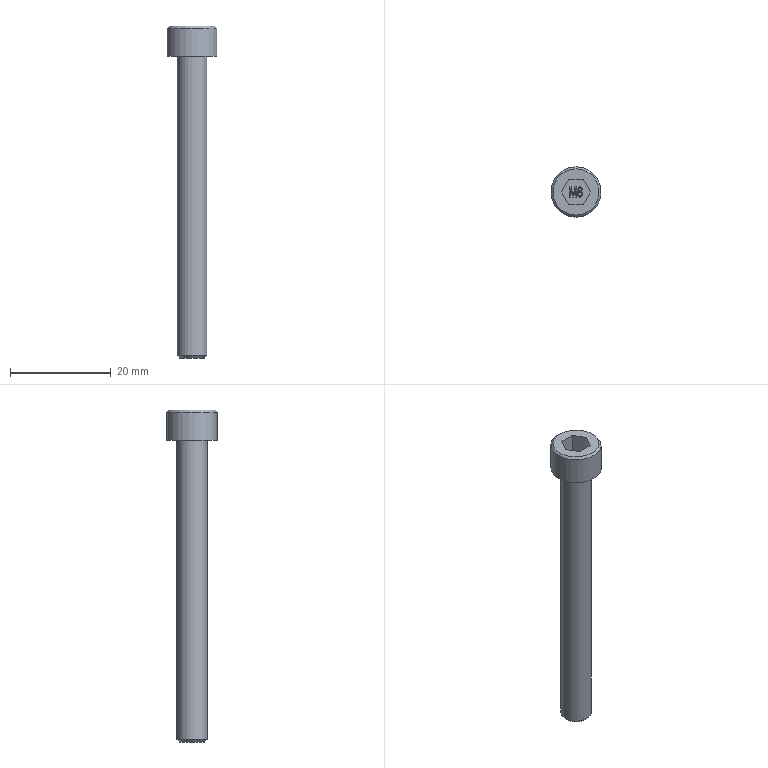Part | STEP file | EM10606000 | 1 solid | 38 faces | box 10 x 10 x 66 mm | volume 2076 mm3 | plane 25 | other 9 | cone 2 | cylinder 2 | commonest cylinder face diameters 6 x1 10 x1